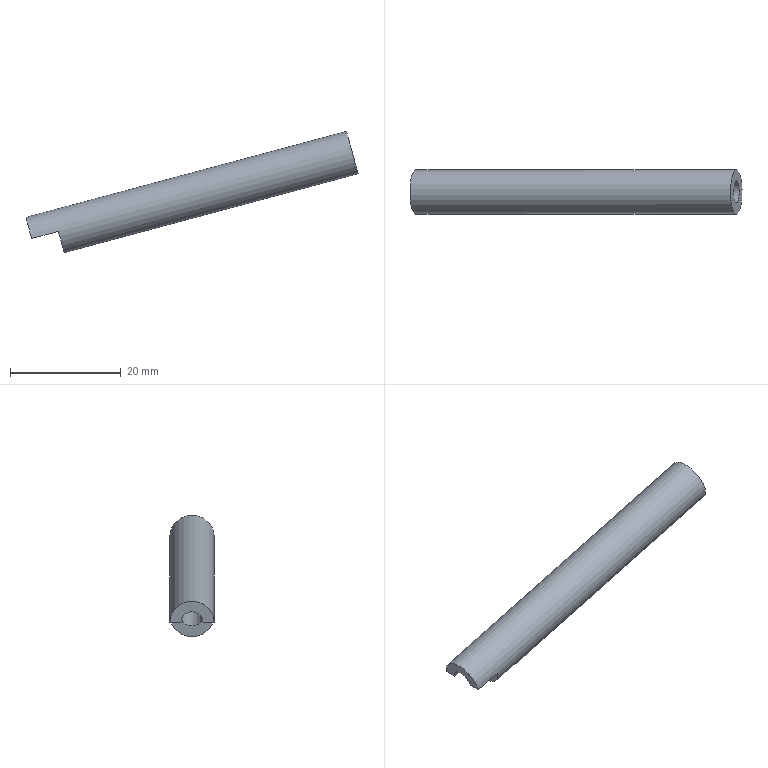Part | NX | features solid 2 | 1 solid | 7 faces | box 60.026 x 8 x 21.962 mm | volume 2167 mm3 | plane 5 | cylinder 2 | commonest cylinder face diameters 4.003 x1 8 x1
STEP:
#1=CARTESIAN_POINT('',(852.68,5.563,-16.417));
#2=VERTEX_POINT('',#1);
#3=CARTESIAN_POINT('',(852.68,13.563,-16.417));
#4=VERTEX_POINT('',#3);
#5=CARTESIAN_POINT('',(852.68,9.563,-16.417));
#6=DIRECTION('',(-0.9659,0.000000134,-0.2588));
#7=DIRECTION('',(0.000000129,1.,0.000000035));
#8=AXIS2_PLACEMENT_3D('',#5,#6,#7);
#9=CIRCLE('',#8,4.);
#10=EDGE_CURVE('',#2,#4,#9,.T.);
#11=ORIENTED_EDGE('',*,*,#10,.T.);
#12=CARTESIAN_POINT('',(852.68,11.565,-16.417));
#13=VERTEX_POINT('',#12);
#14=CARTESIAN_POINT('',(852.68,14.563,-16.417));
#15=DIRECTION('',(-0.000000129,-1.,-0.000000035));
#16=VECTOR('',#15,1000.);
#17=LINE('',#14,#16);
#18=EDGE_CURVE('',#4,#13,#17,.T.);
#19=ORIENTED_EDGE('',*,*,#18,.T.);
#20=CARTESIAN_POINT('',(852.68,7.562,-16.417));
#21=VERTEX_POINT('',#20);
#22=CARTESIAN_POINT('',(852.68,9.563,-16.417));
#23=DIRECTION('',(-0.9659,0.000000134,-0.2588));
#24=DIRECTION('',(0.000000129,1.,0.000000035));
#25=AXIS2_PLACEMENT_3D('',#22,#23,#24);
#26=CIRCLE('',#25,2.002);
#27=EDGE_CURVE('',#21,#13,#26,.T.);
#28=ORIENTED_EDGE('',*,*,#27,.F.);
#29=CARTESIAN_POINT('',(852.68,14.563,-16.417));
#30=DIRECTION('',(-0.000000129,-1.,-0.000000035));
#31=VECTOR('',#30,1000.);
#32=LINE('',#29,#31);
#33=EDGE_CURVE('',#21,#2,#32,.T.);
#34=ORIENTED_EDGE('',*,*,#33,.T.);
#35=EDGE_LOOP('',(#11,#19,#28,#34));
#36=FACE_BOUND('',#35,.T.);
#37=CARTESIAN_POINT('',(852.68,9.563,-16.417));
#38=DIRECTION('',(-0.9659,0.000000134,-0.2588));
#39=DIRECTION('',(0.000000129,1.,0.000000035));
#40=AXIS2_PLACEMENT_3D('',#37,#38,#39);
#41=PLANE('',#40);
#42=ADVANCED_FACE('',(#36),#41,.T.);
#43=ORIENTED_EDGE('',*,*,#10,.F.);
#44=CARTESIAN_POINT('',(857.51,5.563,-15.123));
#45=VERTEX_POINT('',#44);
#46=CARTESIAN_POINT('',(852.68,5.563,-16.417));
#47=DIRECTION('',(0.9659,-0.000000134,0.2588));
#48=VECTOR('',#47,1000.);
#49=LINE('',#46,#48);
#50=EDGE_CURVE('',#2,#45,#49,.T.);
#51=ORIENTED_EDGE('',*,*,#50,.T.);
#52=CARTESIAN_POINT('',(857.51,13.563,-15.123));
#53=VERTEX_POINT('',#52);
#54=CARTESIAN_POINT('',(857.51,9.563,-15.123));
#55=DIRECTION('',(-0.9659,0.000000134,-0.2588));
#56=DIRECTION('',(0.000000129,1.,0.000000035));
#57=AXIS2_PLACEMENT_3D('',#54,#55,#56);
#58=CIRCLE('',#57,4.);
#59=EDGE_CURVE('',#53,#45,#58,.T.);
#60=ORIENTED_EDGE('',*,*,#59,.F.);
#61=CARTESIAN_POINT('',(852.68,13.563,-16.417));
#62=DIRECTION('',(0.9659,-0.000000134,0.2588));
#63=VECTOR('',#62,1000.);
#64=LINE('',#61,#63);
#65=EDGE_CURVE('',#53,#4,#64,.F.);
#66=ORIENTED_EDGE('',*,*,#65,.T.);
#67=EDGE_LOOP('',(#43,#51,#60,#66));
#68=FACE_BOUND('',#67,.T.);
#69=CARTESIAN_POINT('',(910.636,13.563,-0.8879));
#70=VERTEX_POINT('',#69);
#71=CARTESIAN_POINT('',(910.636,9.563,-0.8879));
#72=DIRECTION('',(-0.9659,0.000000134,-0.2588));
#73=DIRECTION('',(0.000000129,1.,0.000000035));
#74=AXIS2_PLACEMENT_3D('',#71,#72,#73);
#75=CIRCLE('',#74,4.);
#76=EDGE_CURVE('',#70,#70,#75,.T.);
#77=ORIENTED_EDGE('',*,*,#76,.T.);
#78=EDGE_LOOP('',(#77));
#79=FACE_BOUND('',#78,.T.);
#80=CARTESIAN_POINT('',(852.68,9.563,-16.417));
#81=DIRECTION('',(0.9659,-0.000000134,0.2588));
#82=DIRECTION('',(-0.000000129,-1.,-0.000000035));
#83=AXIS2_PLACEMENT_3D('',#80,#81,#82);
#84=CYLINDRICAL_SURFACE('',#83,4.);
#85=ADVANCED_FACE('',(#68,#79),#84,.T.);
#86=CARTESIAN_POINT('',(910.636,11.565,-0.8879));
#87=VERTEX_POINT('',#86);
#88=CARTESIAN_POINT('',(910.636,9.563,-0.8879));
#89=DIRECTION('',(-0.9659,0.000000134,-0.2588));
#90=DIRECTION('',(0.000000129,1.,0.000000035));
#91=AXIS2_PLACEMENT_3D('',#88,#89,#90);
#92=CIRCLE('',#91,2.002);
#93=EDGE_CURVE('',#87,#87,#92,.T.);
#94=ORIENTED_EDGE('',*,*,#93,.T.);
#95=EDGE_LOOP('',(#94));
#96=FACE_BOUND('',#95,.T.);
#97=ORIENTED_EDGE('',*,*,#76,.F.);
#98=EDGE_LOOP('',(#97));
#99=FACE_BOUND('',#98,.T.);
#100=CARTESIAN_POINT('',(910.636,9.563,-0.8879));
#101=DIRECTION('',(-0.9659,0.000000134,-0.2588));
#102=DIRECTION('',(0.000000129,1.,0.000000035));
#103=AXIS2_PLACEMENT_3D('',#100,#101,#102);
#104=PLANE('',#103);
#105=ADVANCED_FACE('',(#96,#99),#104,.F.);
#106=CARTESIAN_POINT('',(857.51,7.562,-15.123));
#107=VERTEX_POINT('',#106);
#108=CARTESIAN_POINT('',(852.68,7.562,-16.417));
#109=DIRECTION('',(0.9659,-0.000000134,0.2588));
#110=VECTOR('',#109,1000.);
#111=LINE('',#108,#110);
#112=EDGE_CURVE('',#21,#107,#111,.T.);
#113=ORIENTED_EDGE('',*,*,#112,.F.);
#114=ORIENTED_EDGE('',*,*,#27,.T.);
#115=CARTESIAN_POINT('',(857.51,11.565,-15.123));
#116=VERTEX_POINT('',#115);
#117=CARTESIAN_POINT('',(852.68,11.565,-16.417));
#118=DIRECTION('',(0.9659,-0.000000134,0.2588));
#119=VECTOR('',#118,1000.);
#120=LINE('',#117,#119);
#121=EDGE_CURVE('',#116,#13,#120,.F.);
#122=ORIENTED_EDGE('',*,*,#121,.F.);
#123=CARTESIAN_POINT('',(857.51,9.563,-15.123));
#124=DIRECTION('',(-0.9659,0.000000134,-0.2588));
#125=DIRECTION('',(0.000000129,1.,0.000000035));
#126=AXIS2_PLACEMENT_3D('',#123,#124,#125);
#127=CIRCLE('',#126,2.002);
#128=EDGE_CURVE('',#116,#107,#127,.T.);
#129=ORIENTED_EDGE('',*,*,#128,.T.);
#130=EDGE_LOOP('',(#113,#114,#122,#129));
#131=FACE_BOUND('',#130,.T.);
#132=ORIENTED_EDGE('',*,*,#93,.F.);
#133=EDGE_LOOP('',(#132));
#134=FACE_BOUND('',#133,.T.);
#135=CARTESIAN_POINT('',(852.68,9.563,-16.417));
#136=DIRECTION('',(0.9659,-0.000000134,0.2588));
#137=DIRECTION('',(-0.000000129,-1.,-0.000000035));
#138=AXIS2_PLACEMENT_3D('',#135,#136,#137);
#139=CYLINDRICAL_SURFACE('',#138,2.002);
#140=ADVANCED_FACE('',(#131,#134),#139,.F.);
#141=ORIENTED_EDGE('',*,*,#33,.F.);
#142=ORIENTED_EDGE('',*,*,#112,.T.);
#143=CARTESIAN_POINT('',(857.51,14.563,-15.123));
#144=DIRECTION('',(-0.000000129,-1.,-0.000000035));
#145=VECTOR('',#144,1000.);
#146=LINE('',#143,#145);
#147=EDGE_CURVE('',#45,#107,#146,.F.);
#148=ORIENTED_EDGE('',*,*,#147,.F.);
#149=ORIENTED_EDGE('',*,*,#50,.F.);
#150=EDGE_LOOP('',(#141,#142,#148,#149));
#151=FACE_BOUND('',#150,.T.);
#152=CARTESIAN_POINT('',(852.68,14.563,-16.417));
#153=DIRECTION('',(-0.2588,0.,0.9659));
#154=DIRECTION('',(-0.933,-0.2588,-0.25));
#155=AXIS2_PLACEMENT_3D('',#152,#153,#154);
#156=PLANE('',#155);
#157=ADVANCED_FACE('',(#151),#156,.F.);
#158=CARTESIAN_POINT('',(857.51,14.563,-15.123));
#159=DIRECTION('',(-0.000000129,-1.,-0.000000035));
#160=VECTOR('',#159,1000.);
#161=LINE('',#158,#160);
#162=EDGE_CURVE('',#116,#53,#161,.F.);
#163=ORIENTED_EDGE('',*,*,#162,.F.);
#164=ORIENTED_EDGE('',*,*,#121,.T.);
#165=ORIENTED_EDGE('',*,*,#18,.F.);
#166=ORIENTED_EDGE('',*,*,#65,.F.);
#167=EDGE_LOOP('',(#163,#164,#165,#166));
#168=FACE_BOUND('',#167,.T.);
#169=CARTESIAN_POINT('',(852.68,14.563,-16.417));
#170=DIRECTION('',(-0.2588,0.,0.9659));
#171=DIRECTION('',(-0.933,-0.2588,-0.25));
#172=AXIS2_PLACEMENT_3D('',#169,#170,#171);
#173=PLANE('',#172);
#174=ADVANCED_FACE('',(#168),#173,.F.);
#175=ORIENTED_EDGE('',*,*,#59,.T.);
#176=ORIENTED_EDGE('',*,*,#147,.T.);
#177=ORIENTED_EDGE('',*,*,#128,.F.);
#178=ORIENTED_EDGE('',*,*,#162,.T.);
#179=EDGE_LOOP('',(#175,#176,#177,#178));
#180=FACE_BOUND('',#179,.T.);
#181=CARTESIAN_POINT('',(857.51,9.563,-15.123));
#182=DIRECTION('',(-0.9659,0.000000134,-0.2588));
#183=DIRECTION('',(0.000000129,1.,0.000000035));
#184=AXIS2_PLACEMENT_3D('',#181,#182,#183);
#185=PLANE('',#184);
#186=ADVANCED_FACE('',(#180),#185,.T.);
#187=CLOSED_SHELL('',(#42,#85,#105,#140,#157,#174,#186));
#188=MANIFOLD_SOLID_BREP('',#187);
#189=(LENGTH_UNIT()NAMED_UNIT(*)SI_UNIT(.MILLI.,.METRE.));
#190=UNCERTAINTY_MEASURE_WITH_UNIT(LENGTH_MEASURE(0.00001),#189,'','');
#191=(NAMED_UNIT(*)PLANE_ANGLE_UNIT()SI_UNIT($,.RADIAN.));
#192=(NAMED_UNIT(*)SI_UNIT($,.STERADIAN.)SOLID_ANGLE_UNIT());
#193=(GEOMETRIC_REPRESENTATION_CONTEXT(3)GLOBAL_UNCERTAINTY_ASSIGNED_CONTEXT((#190))GLOBAL_UNIT_ASSIGNED_CONTEXT((#189,#191,#192))REPRESENTATION_CONTEXT('',''));
#194=ADVANCED_BREP_SHAPE_REPRESENTATION('',(#188),#193);